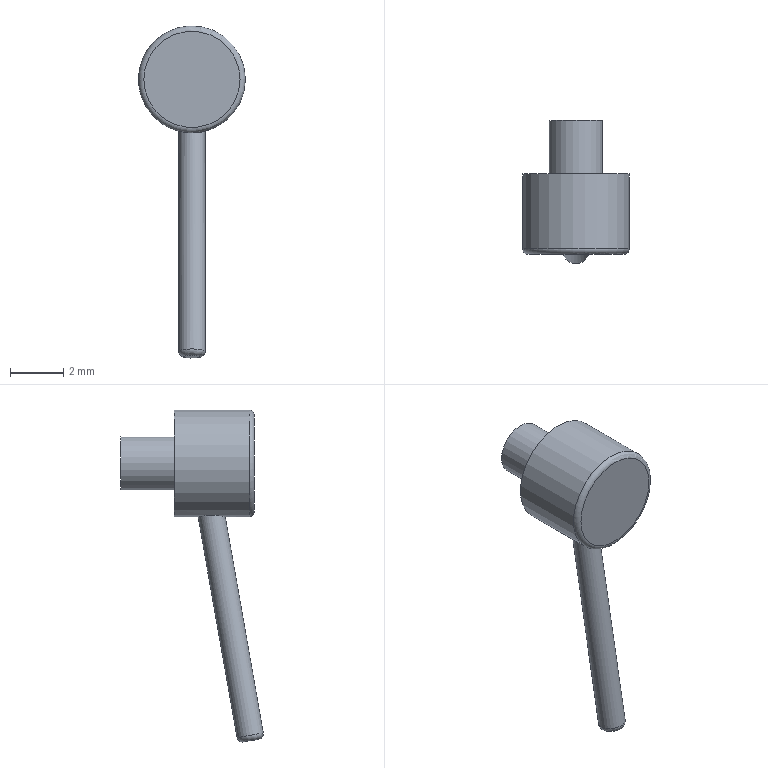Part | STEP file | 1-35.2 | 1 solid | 9 faces | box 4 x 5.337 x 12.426 mm | volume 50.541 mm3 | plane 4 | cylinder 3 | torus 2 | commonest cylinder face diameters 1 x1 2 x1 4 x1
STEP:
#1=CARTESIAN_POINT('',(0.,0.,0.));
#2=DIRECTION('',(0.,0.,1.));
#3=DIRECTION('',(1.,0.,0.));
#4=AXIS2_PLACEMENT_3D('',#1,#2,#3);
#5=CARTESIAN_POINT('',(1.,2.,0.));
#6=VERTEX_POINT('',#5);
#7=CARTESIAN_POINT('',(0.,2.,0.));
#8=DIRECTION('',(0.,-1.,0.));
#9=DIRECTION('',(1.,0.,0.));
#10=AXIS2_PLACEMENT_3D('',#7,#8,#9);
#11=CIRCLE('',#10,1.);
#12=CARTESIAN_POINT('',(-0.2679,2.,0.));
#13=DIRECTION('',(0.,-1.,0.));
#14=DIRECTION('',(1.,0.,0.));
#15=AXIS2_PLACEMENT_3D('',#12,#13,#14);
#16=PLANE('',#15);
#17=CARTESIAN_POINT('',(0.2679,0.));
#18=DIRECTION('',(1.,0.));
#19=AXIS2_PLACEMENT_2D('',#17,#18);
#20=CIRCLE('',#19,1.);
#21=(GEOMETRIC_REPRESENTATION_CONTEXT(2)PARAMETRIC_REPRESENTATION_CONTEXT()REPRESENTATION_CONTEXT('',''));
#22=DEFINITIONAL_REPRESENTATION('',(#20),#21);
#23=PCURVE('',#16,#22);
#24=CARTESIAN_POINT('',(0.,0.,0.));
#25=DIRECTION('',(0.,1.,0.));
#26=DIRECTION('',(1.,0.,0.));
#27=AXIS2_PLACEMENT_3D('',#24,#25,#26);
#28=CYLINDRICAL_SURFACE('',#27,1.);
#29=CARTESIAN_POINT('',(6.283,2.));
#30=DIRECTION('',(-1.,0.));
#31=VECTOR('',#30,1.);
#32=LINE('',#29,#31);
#33=(GEOMETRIC_REPRESENTATION_CONTEXT(2)PARAMETRIC_REPRESENTATION_CONTEXT()REPRESENTATION_CONTEXT('',''));
#34=DEFINITIONAL_REPRESENTATION('',(#32),#33);
#35=PCURVE('',#28,#34);
#36=SURFACE_CURVE('',#11,(#23,#35),.PCURVE_S1.);
#37=EDGE_CURVE('',#6,#6,#36,.T.);
#38=ORIENTED_EDGE('',*,*,#37,.T.);
#39=EDGE_LOOP('',(#38));
#40=FACE_BOUND('',#39,.F.);
#41=ADVANCED_FACE('',(#40),#16,.F.);
#42=CARTESIAN_POINT('',(1.,0.,0.));
#43=VERTEX_POINT('',#42);
#44=CARTESIAN_POINT('',(1.,0.,0.));
#45=DIRECTION('',(0.,1.,0.));
#46=VECTOR('',#45,1.);
#47=LINE('',#44,#46);
#48=CARTESIAN_POINT('',(6.283,0.));
#49=DIRECTION('',(0.,1.));
#50=VECTOR('',#49,1.);
#51=LINE('',#48,#50);
#52=(GEOMETRIC_REPRESENTATION_CONTEXT(2)PARAMETRIC_REPRESENTATION_CONTEXT()REPRESENTATION_CONTEXT('',''));
#53=DEFINITIONAL_REPRESENTATION('',(#51),#52);
#54=PCURVE('',#28,#53);
#55=CARTESIAN_POINT('',(0.,0.));
#56=DIRECTION('',(0.,1.));
#57=VECTOR('',#56,1.);
#58=LINE('',#55,#57);
#59=(GEOMETRIC_REPRESENTATION_CONTEXT(2)PARAMETRIC_REPRESENTATION_CONTEXT()REPRESENTATION_CONTEXT('',''));
#60=DEFINITIONAL_REPRESENTATION('',(#58),#59);
#61=PCURVE('',#28,#60);
#62=SEAM_CURVE('',#47,(#54,#61),.PCURVE_S1.);
#63=EDGE_CURVE('',#43,#6,#62,.T.);
#64=ORIENTED_EDGE('',*,*,#63,.T.);
#65=ORIENTED_EDGE('',*,*,#37,.T.);
#66=ORIENTED_EDGE('',*,*,#63,.F.);
#67=CARTESIAN_POINT('',(0.,0.,0.));
#68=DIRECTION('',(0.,-1.,0.));
#69=DIRECTION('',(1.,0.,0.));
#70=AXIS2_PLACEMENT_3D('',#67,#68,#69);
#71=CIRCLE('',#70,1.);
#72=CARTESIAN_POINT('',(6.283,0.));
#73=DIRECTION('',(-1.,0.));
#74=VECTOR('',#73,1.);
#75=LINE('',#72,#74);
#76=(GEOMETRIC_REPRESENTATION_CONTEXT(2)PARAMETRIC_REPRESENTATION_CONTEXT()REPRESENTATION_CONTEXT('',''));
#77=DEFINITIONAL_REPRESENTATION('',(#75),#76);
#78=PCURVE('',#28,#77);
#79=CARTESIAN_POINT('',(-0.5359,0.,0.));
#80=DIRECTION('',(0.,-1.,0.));
#81=DIRECTION('',(1.,0.,0.));
#82=AXIS2_PLACEMENT_3D('',#79,#80,#81);
#83=PLANE('',#82);
#84=CARTESIAN_POINT('',(0.5359,0.));
#85=DIRECTION('',(1.,0.));
#86=AXIS2_PLACEMENT_2D('',#84,#85);
#87=CIRCLE('',#86,1.);
#88=(GEOMETRIC_REPRESENTATION_CONTEXT(2)PARAMETRIC_REPRESENTATION_CONTEXT()REPRESENTATION_CONTEXT('',''));
#89=DEFINITIONAL_REPRESENTATION('',(#87),#88);
#90=PCURVE('',#83,#89);
#91=SURFACE_CURVE('',#71,(#78,#90),.PCURVE_S1.);
#92=EDGE_CURVE('',#43,#43,#91,.T.);
#93=ORIENTED_EDGE('',*,*,#92,.F.);
#94=EDGE_LOOP('',(#64,#65,#66,#93));
#95=FACE_BOUND('',#94,.T.);
#96=ADVANCED_FACE('',(#95),#28,.T.);
#97=CARTESIAN_POINT('',(2.,0.,0.));
#98=VERTEX_POINT('',#97);
#99=CARTESIAN_POINT('',(0.,0.,0.));
#100=DIRECTION('',(0.,-1.,0.));
#101=DIRECTION('',(1.,0.,0.));
#102=AXIS2_PLACEMENT_3D('',#99,#100,#101);
#103=CIRCLE('',#102,2.);
#104=CARTESIAN_POINT('',(0.5359,0.));
#105=DIRECTION('',(1.,0.));
#106=AXIS2_PLACEMENT_2D('',#104,#105);
#107=CIRCLE('',#106,2.);
#108=(GEOMETRIC_REPRESENTATION_CONTEXT(2)PARAMETRIC_REPRESENTATION_CONTEXT()REPRESENTATION_CONTEXT('',''));
#109=DEFINITIONAL_REPRESENTATION('',(#107),#108);
#110=PCURVE('',#83,#109);
#111=CARTESIAN_POINT('',(0.,0.,0.));
#112=DIRECTION('',(0.,-1.,0.));
#113=DIRECTION('',(1.,0.,0.));
#114=AXIS2_PLACEMENT_3D('',#111,#112,#113);
#115=CYLINDRICAL_SURFACE('',#114,2.);
#116=CARTESIAN_POINT('',(0.,0.));
#117=DIRECTION('',(1.,0.));
#118=VECTOR('',#117,1.);
#119=LINE('',#116,#118);
#120=(GEOMETRIC_REPRESENTATION_CONTEXT(2)PARAMETRIC_REPRESENTATION_CONTEXT()REPRESENTATION_CONTEXT('',''));
#121=DEFINITIONAL_REPRESENTATION('',(#119),#120);
#122=PCURVE('',#115,#121);
#123=SURFACE_CURVE('',#103,(#110,#122),.PCURVE_S1.);
#124=EDGE_CURVE('',#98,#98,#123,.T.);
#125=ORIENTED_EDGE('',*,*,#124,.T.);
#126=EDGE_LOOP('',(#125));
#127=FACE_BOUND('',#126,.F.);
#128=ORIENTED_EDGE('',*,*,#92,.F.);
#129=EDGE_LOOP('',(#128));
#130=FACE_BOUND('',#129,.F.);
#131=ADVANCED_FACE('',(#127,#130),#83,.F.);
#132=CARTESIAN_POINT('',(1.8,-3.,0.));
#133=VERTEX_POINT('',#132);
#134=CARTESIAN_POINT('',(0.,-3.,0.));
#135=DIRECTION('',(0.,1.,0.));
#136=DIRECTION('',(1.,0.,0.));
#137=AXIS2_PLACEMENT_3D('',#134,#135,#136);
#138=CIRCLE('',#137,1.8);
#139=CARTESIAN_POINT('',(-0.5359,-3.,0.));
#140=DIRECTION('',(0.,-1.,0.));
#141=DIRECTION('',(1.,0.,0.));
#142=AXIS2_PLACEMENT_3D('',#139,#140,#141);
#143=PLANE('',#142);
#144=CARTESIAN_POINT('',(2.336,0.));
#145=CARTESIAN_POINT('',(2.336,-3.118));
#146=CARTESIAN_POINT('',(-0.3641,-1.559));
#147=CARTESIAN_POINT('',(-3.064,0.));
#148=CARTESIAN_POINT('',(-0.3641,1.559));
#149=CARTESIAN_POINT('',(2.336,3.118));
#150=CARTESIAN_POINT('',(2.336,0.));
#151=(BOUNDED_CURVE()B_SPLINE_CURVE(2,(#144,#145,#146,#147,#148,#149,#150),.UNSPECIFIED.,.T.,.F.)B_SPLINE_CURVE_WITH_KNOTS((1,2,2,2,2,1),(-2.094,0.,2.094,4.189,6.283,8.378),.UNSPECIFIED.)CURVE()GEOMETRIC_REPRESENTATION_ITEM()RATIONAL_B_SPLINE_CURVE((1.,0.5,1.,0.5,1.,0.5,1.))REPRESENTATION_ITEM(''));
#152=(GEOMETRIC_REPRESENTATION_CONTEXT(2)PARAMETRIC_REPRESENTATION_CONTEXT()REPRESENTATION_CONTEXT('',''));
#153=DEFINITIONAL_REPRESENTATION('',(#151),#152);
#154=PCURVE('',#143,#153);
#155=CARTESIAN_POINT('',(0.,-2.8,0.));
#156=DIRECTION('',(0.,-1.,0.));
#157=DIRECTION('',(1.,0.,0.));
#158=AXIS2_PLACEMENT_3D('',#155,#156,#157);
#159=TOROIDAL_SURFACE('',#158,1.8,0.2);
#160=CARTESIAN_POINT('',(6.283,1.571));
#161=DIRECTION('',(-1.,0.));
#162=VECTOR('',#161,1.);
#163=LINE('',#160,#162);
#164=(GEOMETRIC_REPRESENTATION_CONTEXT(2)PARAMETRIC_REPRESENTATION_CONTEXT()REPRESENTATION_CONTEXT('',''));
#165=DEFINITIONAL_REPRESENTATION('',(#163),#164);
#166=PCURVE('',#159,#165);
#167=SURFACE_CURVE('',#138,(#154,#166),.PCURVE_S1.);
#168=EDGE_CURVE('',#133,#133,#167,.T.);
#169=ORIENTED_EDGE('',*,*,#168,.F.);
#170=EDGE_LOOP('',(#169));
#171=FACE_BOUND('',#170,.T.);
#172=ADVANCED_FACE('',(#171),#143,.T.);
#173=CARTESIAN_POINT('',(2.,-2.8,0.));
#174=VERTEX_POINT('',#173);
#175=CARTESIAN_POINT('',(1.8,-2.8,0.));
#176=DIRECTION('',(0.,0.,1.));
#177=DIRECTION('',(0.,-1.,0.));
#178=AXIS2_PLACEMENT_3D('',#175,#176,#177);
#179=CIRCLE('',#178,0.2);
#180=CARTESIAN_POINT('',(0.,1.571));
#181=DIRECTION('',(0.,-1.));
#182=VECTOR('',#181,1.);
#183=LINE('',#180,#182);
#184=(GEOMETRIC_REPRESENTATION_CONTEXT(2)PARAMETRIC_REPRESENTATION_CONTEXT()REPRESENTATION_CONTEXT('',''));
#185=DEFINITIONAL_REPRESENTATION('',(#183),#184);
#186=PCURVE('',#159,#185);
#187=CARTESIAN_POINT('',(6.283,1.571));
#188=DIRECTION('',(0.,-1.));
#189=VECTOR('',#188,1.);
#190=LINE('',#187,#189);
#191=(GEOMETRIC_REPRESENTATION_CONTEXT(2)PARAMETRIC_REPRESENTATION_CONTEXT()REPRESENTATION_CONTEXT('',''));
#192=DEFINITIONAL_REPRESENTATION('',(#190),#191);
#193=PCURVE('',#159,#192);
#194=SEAM_CURVE('',#179,(#186,#193),.PCURVE_S1.);
#195=EDGE_CURVE('',#133,#174,#194,.T.);
#196=ORIENTED_EDGE('',*,*,#195,.T.);
#197=CARTESIAN_POINT('',(0.,-2.8,0.));
#198=DIRECTION('',(0.,1.,0.));
#199=DIRECTION('',(1.,0.,0.));
#200=AXIS2_PLACEMENT_3D('',#197,#198,#199);
#201=CIRCLE('',#200,2.);
#202=CARTESIAN_POINT('',(6.283,0.));
#203=DIRECTION('',(-1.,0.));
#204=VECTOR('',#203,1.);
#205=LINE('',#202,#204);
#206=(GEOMETRIC_REPRESENTATION_CONTEXT(2)PARAMETRIC_REPRESENTATION_CONTEXT()REPRESENTATION_CONTEXT('',''));
#207=DEFINITIONAL_REPRESENTATION('',(#205),#206);
#208=PCURVE('',#159,#207);
#209=CARTESIAN_POINT('',(6.283,2.8));
#210=DIRECTION('',(-1.,0.));
#211=VECTOR('',#210,1.);
#212=LINE('',#209,#211);
#213=(GEOMETRIC_REPRESENTATION_CONTEXT(2)PARAMETRIC_REPRESENTATION_CONTEXT()REPRESENTATION_CONTEXT('',''));
#214=DEFINITIONAL_REPRESENTATION('',(#212),#213);
#215=PCURVE('',#115,#214);
#216=SURFACE_CURVE('',#201,(#208,#215),.PCURVE_S1.);
#217=EDGE_CURVE('',#174,#174,#216,.T.);
#218=ORIENTED_EDGE('',*,*,#217,.F.);
#219=ORIENTED_EDGE('',*,*,#195,.F.);
#220=ORIENTED_EDGE('',*,*,#168,.T.);
#221=EDGE_LOOP('',(#196,#218,#219,#220));
#222=FACE_BOUND('',#221,.T.);
#223=ADVANCED_FACE('',(#222),#159,.T.);
#224=ORIENTED_EDGE('',*,*,#124,.T.);
#225=CARTESIAN_POINT('',(2.,0.,0.));
#226=DIRECTION('',(0.,-1.,0.));
#227=VECTOR('',#226,1.);
#228=LINE('',#225,#227);
#229=CARTESIAN_POINT('',(6.283,0.));
#230=DIRECTION('',(0.,1.));
#231=VECTOR('',#230,1.);
#232=LINE('',#229,#231);
#233=(GEOMETRIC_REPRESENTATION_CONTEXT(2)PARAMETRIC_REPRESENTATION_CONTEXT()REPRESENTATION_CONTEXT('',''));
#234=DEFINITIONAL_REPRESENTATION('',(#232),#233);
#235=PCURVE('',#115,#234);
#236=CARTESIAN_POINT('',(0.,0.));
#237=DIRECTION('',(0.,1.));
#238=VECTOR('',#237,1.);
#239=LINE('',#236,#238);
#240=(GEOMETRIC_REPRESENTATION_CONTEXT(2)PARAMETRIC_REPRESENTATION_CONTEXT()REPRESENTATION_CONTEXT('',''));
#241=DEFINITIONAL_REPRESENTATION('',(#239),#240);
#242=PCURVE('',#115,#241);
#243=SEAM_CURVE('',#228,(#235,#242),.PCURVE_S1.);
#244=EDGE_CURVE('',#98,#174,#243,.T.);
#245=ORIENTED_EDGE('',*,*,#244,.T.);
#246=ORIENTED_EDGE('',*,*,#217,.T.);
#247=ORIENTED_EDGE('',*,*,#244,.F.);
#248=EDGE_LOOP('',(#224,#245,#246,#247));
#249=FACE_BOUND('',#248,.T.);
#250=CARTESIAN_POINT('',(-0.5,-1.389,-1.936));
#251=VERTEX_POINT('',#250);
#252=CARTESIAN_POINT('',(-0.5,-1.389,-1.936));
#253=CARTESIAN_POINT('',(-0.5,-1.309,-1.936));
#254=CARTESIAN_POINT('',(-0.445,-1.071,-1.951));
#255=CARTESIAN_POINT('',(-0.2312,-0.9214,-1.993));
#256=CARTESIAN_POINT('',(0.147,-0.8642,-2.007));
#257=CARTESIAN_POINT('',(0.3709,-0.9796,-1.967));
#258=CARTESIAN_POINT('',(0.5988,-1.522,-1.913));
#259=CARTESIAN_POINT('',(0.3591,-1.908,-2.));
#260=CARTESIAN_POINT('',(-0.18,-1.908,-2.));
#261=CARTESIAN_POINT('',(-0.429,-1.75,-1.955));
#262=CARTESIAN_POINT('',(-0.5,-1.479,-1.936));
#263=CARTESIAN_POINT('',(-0.5,-1.389,-1.936));
#264=B_SPLINE_CURVE_WITH_KNOTS('',3,(#252,#253,#254,#255,#256,#257,#258,#259,#260,#261,#262,#263),.UNSPECIFIED.,.T.,.F.,(1,3,1,2,2,2,1,3,1),(-0.3333,0.,0.3001,0.9002,1.771,3.101,3.768,4.101,4.401),.UNSPECIFIED.);
#265=CARTESIAN_POINT('',(4.46,1.389));
#266=CARTESIAN_POINT('',(4.46,1.364));
#267=CARTESIAN_POINT('',(4.462,1.315));
#268=CARTESIAN_POINT('',(4.47,1.243));
#269=CARTESIAN_POINT('',(4.483,1.174));
#270=CARTESIAN_POINT('',(4.502,1.111));
#271=CARTESIAN_POINT('',(4.525,1.054));
#272=CARTESIAN_POINT('',(4.552,1.004));
#273=CARTESIAN_POINT('',(4.583,0.962));
#274=CARTESIAN_POINT('',(4.616,0.9291));
#275=CARTESIAN_POINT('',(4.65,0.9058));
#276=CARTESIAN_POINT('',(4.686,0.8932));
#277=CARTESIAN_POINT('',(4.722,0.8909));
#278=CARTESIAN_POINT('',(4.757,0.8984));
#279=CARTESIAN_POINT('',(4.791,0.9152));
#280=CARTESIAN_POINT('',(4.824,0.9411));
#281=CARTESIAN_POINT('',(4.855,0.9756));
#282=CARTESIAN_POINT('',(4.882,1.018));
#283=CARTESIAN_POINT('',(4.907,1.069));
#284=CARTESIAN_POINT('',(4.929,1.127));
#285=CARTESIAN_POINT('',(4.946,1.193));
#286=CARTESIAN_POINT('',(4.958,1.264));
#287=CARTESIAN_POINT('',(4.964,1.334));
#288=CARTESIAN_POINT('',(4.966,1.405));
#289=CARTESIAN_POINT('',(4.962,1.474));
#290=CARTESIAN_POINT('',(4.954,1.541));
#291=CARTESIAN_POINT('',(4.941,1.606));
#292=CARTESIAN_POINT('',(4.925,1.667));
#293=CARTESIAN_POINT('',(4.905,1.723));
#294=CARTESIAN_POINT('',(4.881,1.773));
#295=CARTESIAN_POINT('',(4.855,1.817));
#296=CARTESIAN_POINT('',(4.825,1.854));
#297=CARTESIAN_POINT('',(4.794,1.882));
#298=CARTESIAN_POINT('',(4.759,1.901));
#299=CARTESIAN_POINT('',(4.723,1.909));
#300=CARTESIAN_POINT('',(4.685,1.906));
#301=CARTESIAN_POINT('',(4.649,1.892));
#302=CARTESIAN_POINT('',(4.614,1.866));
#303=CARTESIAN_POINT('',(4.581,1.831));
#304=CARTESIAN_POINT('',(4.551,1.787));
#305=CARTESIAN_POINT('',(4.524,1.735));
#306=CARTESIAN_POINT('',(4.502,1.675));
#307=CARTESIAN_POINT('',(4.483,1.609));
#308=CARTESIAN_POINT('',(4.47,1.539));
#309=CARTESIAN_POINT('',(4.462,1.464));
#310=CARTESIAN_POINT('',(4.46,1.414));
#311=CARTESIAN_POINT('',(4.46,1.389));
#312=B_SPLINE_CURVE_WITH_KNOTS('',3,(#265,#266,#267,#268,#269,#270,#271,#272,#273,#274,#275,#276,#277,#278,#279,#280,#281,#282,#283,#284,#285,#286,#287,#288,#289,#290,#291,#292,#293,#294,#295,#296,#297,#298,#299,#300,#301,#302,#303,#304,#305,#306,#307,#308,#309,#310,#311),.UNSPECIFIED.,.T.,.F.,(4,1,1,1,1,1,1,1,1,1,1,1,1,1,1,1,1,1,1,1,1,1,1,1,1,1,1,1,1,1,1,1,1,1,1,1,1,1,1,1,1,1,1,1,4),(0.,0.09321,0.1864,0.2796,0.3729,0.4661,0.5593,0.6525,0.7457,0.8389,0.9321,1.025,1.119,1.212,1.305,1.398,1.491,1.585,1.678,1.771,1.864,1.957,2.051,2.144,2.237,2.33,2.424,2.517,2.61,2.703,2.796,2.89,2.983,3.076,3.169,3.262,3.356,3.449,3.542,3.635,3.729,3.822,3.915,4.008,4.101),.QUASI_UNIFORM_KNOTS.);
#313=(GEOMETRIC_REPRESENTATION_CONTEXT(2)PARAMETRIC_REPRESENTATION_CONTEXT()REPRESENTATION_CONTEXT('',''));
#314=DEFINITIONAL_REPRESENTATION('',(#312),#313);
#315=PCURVE('',#115,#314);
#316=CARTESIAN_POINT('',(0.,-0.3263,4.089));
#317=DIRECTION('',(0.,-0.1736,-0.9848));
#318=DIRECTION('',(-1.,0.,0.));
#319=AXIS2_PLACEMENT_3D('',#316,#317,#318);
#320=CYLINDRICAL_SURFACE('',#319,0.5);
#321=CARTESIAN_POINT('',(0.,6.119));
#322=CARTESIAN_POINT('',(0.04857,6.114));
#323=CARTESIAN_POINT('',(0.146,6.107));
#324=CARTESIAN_POINT('',(0.2926,6.098));
#325=CARTESIAN_POINT('',(0.439,6.092));
#326=CARTESIAN_POINT('',(0.5854,6.089));
#327=CARTESIAN_POINT('',(0.7324,6.088));
#328=CARTESIAN_POINT('',(0.8799,6.088));
#329=CARTESIAN_POINT('',(1.028,6.09));
#330=CARTESIAN_POINT('',(1.175,6.092));
#331=CARTESIAN_POINT('',(1.321,6.094));
#332=CARTESIAN_POINT('',(1.467,6.095));
#333=CARTESIAN_POINT('',(1.61,6.095));
#334=CARTESIAN_POINT('',(1.751,6.093));
#335=CARTESIAN_POINT('',(1.891,6.092));
#336=CARTESIAN_POINT('',(2.031,6.09));
#337=CARTESIAN_POINT('',(2.17,6.088));
#338=CARTESIAN_POINT('',(2.311,6.088));
#339=CARTESIAN_POINT('',(2.453,6.088));
#340=CARTESIAN_POINT('',(2.596,6.09));
#341=CARTESIAN_POINT('',(2.745,6.094));
#342=CARTESIAN_POINT('',(2.892,6.101));
#343=CARTESIAN_POINT('',(3.033,6.111));
#344=CARTESIAN_POINT('',(3.172,6.124));
#345=CARTESIAN_POINT('',(3.307,6.139));
#346=CARTESIAN_POINT('',(3.442,6.155));
#347=CARTESIAN_POINT('',(3.576,6.172));
#348=CARTESIAN_POINT('',(3.709,6.19));
#349=CARTESIAN_POINT('',(3.842,6.207));
#350=CARTESIAN_POINT('',(3.976,6.223));
#351=CARTESIAN_POINT('',(4.11,6.238));
#352=CARTESIAN_POINT('',(4.246,6.251));
#353=CARTESIAN_POINT('',(4.384,6.261));
#354=CARTESIAN_POINT('',(4.525,6.269));
#355=CARTESIAN_POINT('',(4.671,6.272));
#356=CARTESIAN_POINT('',(4.822,6.271));
#357=CARTESIAN_POINT('',(4.97,6.264));
#358=CARTESIAN_POINT('',(5.116,6.254));
#359=CARTESIAN_POINT('',(5.261,6.24));
#360=CARTESIAN_POINT('',(5.406,6.223));
#361=CARTESIAN_POINT('',(5.551,6.205));
#362=CARTESIAN_POINT('',(5.695,6.186));
#363=CARTESIAN_POINT('',(5.84,6.168));
#364=CARTESIAN_POINT('',(5.987,6.149));
#365=CARTESIAN_POINT('',(6.134,6.133));
#366=CARTESIAN_POINT('',(6.234,6.123));
#367=CARTESIAN_POINT('',(6.283,6.119));
#368=B_SPLINE_CURVE_WITH_KNOTS('',3,(#321,#322,#323,#324,#325,#326,#327,#328,#329,#330,#331,#332,#333,#334,#335,#336,#337,#338,#339,#340,#341,#342,#343,#344,#345,#346,#347,#348,#349,#350,#351,#352,#353,#354,#355,#356,#357,#358,#359,#360,#361,#362,#363,#364,#365,#366,#367),.UNSPECIFIED.,.F.,.F.,(4,1,1,1,1,1,1,1,1,1,1,1,1,1,1,1,1,1,1,1,1,1,1,1,1,1,1,1,1,1,1,1,1,1,1,1,1,1,1,1,1,1,1,1,4),(0.,0.09321,0.1864,0.2796,0.3729,0.4661,0.5593,0.6525,0.7457,0.8389,0.9321,1.025,1.119,1.212,1.305,1.398,1.491,1.585,1.678,1.771,1.864,1.957,2.051,2.144,2.237,2.33,2.424,2.517,2.61,2.703,2.796,2.89,2.983,3.076,3.169,3.262,3.356,3.449,3.542,3.635,3.729,3.822,3.915,4.008,4.101),.QUASI_UNIFORM_KNOTS.);
#369=(GEOMETRIC_REPRESENTATION_CONTEXT(2)PARAMETRIC_REPRESENTATION_CONTEXT()REPRESENTATION_CONTEXT('',''));
#370=DEFINITIONAL_REPRESENTATION('',(#368),#369);
#371=PCURVE('',#320,#370);
#372=SURFACE_CURVE('',#264,(#315,#371),.PCURVE_S1.);
#373=EDGE_CURVE('',#251,#251,#372,.T.);
#374=ORIENTED_EDGE('',*,*,#373,.F.);
#375=EDGE_LOOP('',(#374));
#376=FACE_BOUND('',#375,.T.);
#377=ADVANCED_FACE('',(#249,#376),#115,.T.);
#378=CARTESIAN_POINT('',(-0.5,-2.841,-10.174));
#379=VERTEX_POINT('',#378);
#380=CARTESIAN_POINT('',(-0.5,-2.841,-10.174));
#381=DIRECTION('',(0.,0.1736,0.9848));
#382=VECTOR('',#381,1.);
#383=LINE('',#380,#382);
#384=CARTESIAN_POINT('',(6.283,14.483));
#385=DIRECTION('',(0.,-1.));
#386=VECTOR('',#385,1.);
#387=LINE('',#384,#386);
#388=(GEOMETRIC_REPRESENTATION_CONTEXT(2)PARAMETRIC_REPRESENTATION_CONTEXT()REPRESENTATION_CONTEXT('',''));
#389=DEFINITIONAL_REPRESENTATION('',(#387),#388);
#390=PCURVE('',#320,#389);
#391=CARTESIAN_POINT('',(0.,14.483));
#392=DIRECTION('',(0.,-1.));
#393=VECTOR('',#392,1.);
#394=LINE('',#391,#393);
#395=(GEOMETRIC_REPRESENTATION_CONTEXT(2)PARAMETRIC_REPRESENTATION_CONTEXT()REPRESENTATION_CONTEXT('',''));
#396=DEFINITIONAL_REPRESENTATION('',(#394),#395);
#397=PCURVE('',#320,#396);
#398=SEAM_CURVE('',#383,(#390,#397),.PCURVE_S1.);
#399=EDGE_CURVE('',#379,#251,#398,.T.);
#400=ORIENTED_EDGE('',*,*,#399,.F.);
#401=CARTESIAN_POINT('',(0.,-2.841,-10.174));
#402=DIRECTION('',(0.,0.1736,0.9848));
#403=DIRECTION('',(-1.,0.,0.));
#404=AXIS2_PLACEMENT_3D('',#401,#402,#403);
#405=CIRCLE('',#404,0.5);
#406=CARTESIAN_POINT('',(6.283,14.483));
#407=DIRECTION('',(-1.,0.));
#408=VECTOR('',#407,1.);
#409=LINE('',#406,#408);
#410=(GEOMETRIC_REPRESENTATION_CONTEXT(2)PARAMETRIC_REPRESENTATION_CONTEXT()REPRESENTATION_CONTEXT('',''));
#411=DEFINITIONAL_REPRESENTATION('',(#409),#410);
#412=PCURVE('',#320,#411);
#413=CARTESIAN_POINT('',(0.,-2.841,-10.174));
#414=DIRECTION('',(0.,-0.1736,-0.9848));
#415=DIRECTION('',(-1.,0.,0.));
#416=AXIS2_PLACEMENT_3D('',#413,#414,#415);
#417=TOROIDAL_SURFACE('',#416,0.3,0.2);
#418=CARTESIAN_POINT('',(6.283,0.));
#419=DIRECTION('',(-1.,0.));
#420=VECTOR('',#419,1.);
#421=LINE('',#418,#420);
#422=(GEOMETRIC_REPRESENTATION_CONTEXT(2)PARAMETRIC_REPRESENTATION_CONTEXT()REPRESENTATION_CONTEXT('',''));
#423=DEFINITIONAL_REPRESENTATION('',(#421),#422);
#424=PCURVE('',#417,#423);
#425=SURFACE_CURVE('',#405,(#412,#424),.PCURVE_S1.);
#426=EDGE_CURVE('',#379,#379,#425,.T.);
#427=ORIENTED_EDGE('',*,*,#426,.T.);
#428=ORIENTED_EDGE('',*,*,#399,.T.);
#429=ORIENTED_EDGE('',*,*,#373,.T.);
#430=EDGE_LOOP('',(#400,#427,#428,#429));
#431=FACE_BOUND('',#430,.T.);
#432=ADVANCED_FACE('',(#431),#320,.T.);
#433=CARTESIAN_POINT('',(-0.3,-2.876,-10.371));
#434=VERTEX_POINT('',#433);
#435=CARTESIAN_POINT('',(0.,-2.876,-10.371));
#436=DIRECTION('',(0.,0.1736,0.9848));
#437=DIRECTION('',(-1.,0.,0.));
#438=AXIS2_PLACEMENT_3D('',#435,#436,#437);
#439=CIRCLE('',#438,0.3);
#440=CARTESIAN_POINT('',(0.,-2.876,-10.371));
#441=DIRECTION('',(0.,-0.1736,-0.9848));
#442=DIRECTION('',(1.,0.,0.));
#443=AXIS2_PLACEMENT_3D('',#440,#441,#442);
#444=PLANE('',#443);
#445=CARTESIAN_POINT('',(-0.3,0.));
#446=CARTESIAN_POINT('',(-0.3,0.5196));
#447=CARTESIAN_POINT('',(0.15,0.2598));
#448=CARTESIAN_POINT('',(0.6,0.));
#449=CARTESIAN_POINT('',(0.15,-0.2598));
#450=CARTESIAN_POINT('',(-0.3,-0.5196));
#451=CARTESIAN_POINT('',(-0.3,0.));
#452=(BOUNDED_CURVE()B_SPLINE_CURVE(2,(#445,#446,#447,#448,#449,#450,#451),.UNSPECIFIED.,.T.,.F.)B_SPLINE_CURVE_WITH_KNOTS((1,2,2,2,2,1),(-2.094,0.,2.094,4.189,6.283,8.378),.UNSPECIFIED.)CURVE()GEOMETRIC_REPRESENTATION_ITEM()RATIONAL_B_SPLINE_CURVE((1.,0.5,1.,0.5,1.,0.5,1.))REPRESENTATION_ITEM(''));
#453=(GEOMETRIC_REPRESENTATION_CONTEXT(2)PARAMETRIC_REPRESENTATION_CONTEXT()REPRESENTATION_CONTEXT('',''));
#454=DEFINITIONAL_REPRESENTATION('',(#452),#453);
#455=PCURVE('',#444,#454);
#456=CARTESIAN_POINT('',(6.283,1.571));
#457=DIRECTION('',(-1.,0.));
#458=VECTOR('',#457,1.);
#459=LINE('',#456,#458);
#460=(GEOMETRIC_REPRESENTATION_CONTEXT(2)PARAMETRIC_REPRESENTATION_CONTEXT()REPRESENTATION_CONTEXT('',''));
#461=DEFINITIONAL_REPRESENTATION('',(#459),#460);
#462=PCURVE('',#417,#461);
#463=SURFACE_CURVE('',#439,(#455,#462),.PCURVE_S1.);
#464=EDGE_CURVE('',#434,#434,#463,.T.);
#465=ORIENTED_EDGE('',*,*,#464,.F.);
#466=EDGE_LOOP('',(#465));
#467=FACE_BOUND('',#466,.T.);
#468=ADVANCED_FACE('',(#467),#444,.T.);
#469=CARTESIAN_POINT('',(-0.3,-2.841,-10.174));
#470=DIRECTION('',(0.,-0.9848,0.1736));
#471=DIRECTION('',(-1.,0.,0.));
#472=AXIS2_PLACEMENT_3D('',#469,#470,#471);
#473=CIRCLE('',#472,0.2);
#474=CARTESIAN_POINT('',(0.,0.));
#475=DIRECTION('',(0.,1.));
#476=VECTOR('',#475,1.);
#477=LINE('',#474,#476);
#478=(GEOMETRIC_REPRESENTATION_CONTEXT(2)PARAMETRIC_REPRESENTATION_CONTEXT()REPRESENTATION_CONTEXT('',''));
#479=DEFINITIONAL_REPRESENTATION('',(#477),#478);
#480=PCURVE('',#417,#479);
#481=CARTESIAN_POINT('',(6.283,0.));
#482=DIRECTION('',(0.,1.));
#483=VECTOR('',#482,1.);
#484=LINE('',#481,#483);
#485=(GEOMETRIC_REPRESENTATION_CONTEXT(2)PARAMETRIC_REPRESENTATION_CONTEXT()REPRESENTATION_CONTEXT('',''));
#486=DEFINITIONAL_REPRESENTATION('',(#484),#485);
#487=PCURVE('',#417,#486);
#488=SEAM_CURVE('',#473,(#480,#487),.PCURVE_S1.);
#489=EDGE_CURVE('',#379,#434,#488,.T.);
#490=ORIENTED_EDGE('',*,*,#489,.F.);
#491=ORIENTED_EDGE('',*,*,#426,.F.);
#492=ORIENTED_EDGE('',*,*,#489,.T.);
#493=ORIENTED_EDGE('',*,*,#464,.T.);
#494=EDGE_LOOP('',(#490,#491,#492,#493));
#495=FACE_BOUND('',#494,.T.);
#496=ADVANCED_FACE('',(#495),#417,.T.);
#497=CLOSED_SHELL('',(#41,#96,#131,#172,#223,#377,#432,#468,#496));
#498=MANIFOLD_SOLID_BREP('',#497);
#499=(LENGTH_UNIT()NAMED_UNIT(*)SI_UNIT(.MILLI.,.METRE.));
#500=UNCERTAINTY_MEASURE_WITH_UNIT(LENGTH_MEASURE(0.0005),#499,'','');
#501=(NAMED_UNIT(*)PLANE_ANGLE_UNIT()SI_UNIT($,.RADIAN.));
#502=(NAMED_UNIT(*)SI_UNIT($,.STERADIAN.)SOLID_ANGLE_UNIT());
#503=(GEOMETRIC_REPRESENTATION_CONTEXT(3)GLOBAL_UNCERTAINTY_ASSIGNED_CONTEXT((#500))GLOBAL_UNIT_ASSIGNED_CONTEXT((#499,#501,#502))REPRESENTATION_CONTEXT('',''));
#504=ADVANCED_BREP_SHAPE_REPRESENTATION('',(#4,#498),#503);